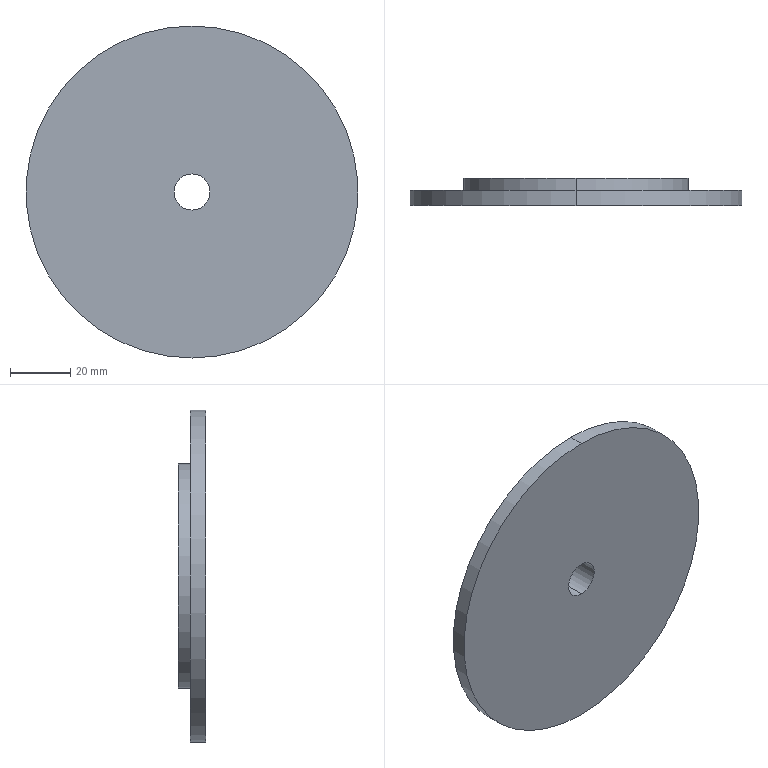Part | NX | features BREP 1 | 1 solid | 9 faces | box 110 x 9 x 110 mm | volume 63935 mm3 | cylinder 6 | plane 3 | commonest cylinder face diameters 12 x2 74.5 x2 110 x2
STEP:
#1=CARTESIAN_POINT('',(0.,6.5,37.25));
#2=VERTEX_POINT('',#1);
#3=CARTESIAN_POINT('',(0.,6.5,-37.25));
#4=VERTEX_POINT('',#3);
#5=CARTESIAN_POINT('',(0.,6.5,0.));
#6=DIRECTION('',(0.,1.,0.));
#7=DIRECTION('',(0.,0.,1.));
#8=AXIS2_PLACEMENT_3D('',#5,#6,#7);
#9=CIRCLE('',#8,37.25);
#10=EDGE_CURVE('',#2,#4,#9,.T.);
#11=ORIENTED_EDGE('',*,*,#10,.F.);
#12=CARTESIAN_POINT('',(0.,2.5,37.25));
#13=VERTEX_POINT('',#12);
#14=CARTESIAN_POINT('',(0.,6.5,37.25));
#15=DIRECTION('',(0.,-1.,0.));
#16=VECTOR('',#15,1000.);
#17=LINE('',#14,#16);
#18=EDGE_CURVE('',#13,#2,#17,.F.);
#19=ORIENTED_EDGE('',*,*,#18,.F.);
#20=CARTESIAN_POINT('',(0.,2.5,-37.25));
#21=VERTEX_POINT('',#20);
#22=CARTESIAN_POINT('',(0.,2.5,0.));
#23=DIRECTION('',(0.,1.,0.));
#24=DIRECTION('',(0.,0.,1.));
#25=AXIS2_PLACEMENT_3D('',#22,#23,#24);
#26=CIRCLE('',#25,37.25);
#27=EDGE_CURVE('',#13,#21,#26,.T.);
#28=ORIENTED_EDGE('',*,*,#27,.T.);
#29=CARTESIAN_POINT('',(0.,6.5,-37.25));
#30=DIRECTION('',(0.,-1.,0.));
#31=VECTOR('',#30,1000.);
#32=LINE('',#29,#31);
#33=EDGE_CURVE('',#21,#4,#32,.F.);
#34=ORIENTED_EDGE('',*,*,#33,.T.);
#35=EDGE_LOOP('',(#11,#19,#28,#34));
#36=FACE_BOUND('',#35,.T.);
#37=CARTESIAN_POINT('',(0.,6.5,0.));
#38=DIRECTION('',(0.,-1.,0.));
#39=DIRECTION('',(0.,0.,1.));
#40=AXIS2_PLACEMENT_3D('',#37,#38,#39);
#41=CYLINDRICAL_SURFACE('',#40,37.25);
#42=ADVANCED_FACE('',(#36),#41,.T.);
#43=CARTESIAN_POINT('',(0.,6.5,-6.));
#44=VERTEX_POINT('',#43);
#45=CARTESIAN_POINT('',(0.,6.5,6.));
#46=VERTEX_POINT('',#45);
#47=CARTESIAN_POINT('',(0.,6.5,0.));
#48=DIRECTION('',(0.,1.,0.));
#49=DIRECTION('',(0.,0.,1.));
#50=AXIS2_PLACEMENT_3D('',#47,#48,#49);
#51=CIRCLE('',#50,6.);
#52=EDGE_CURVE('',#44,#46,#51,.T.);
#53=ORIENTED_EDGE('',*,*,#52,.T.);
#54=CARTESIAN_POINT('',(0.,-2.5,6.));
#55=VERTEX_POINT('',#54);
#56=CARTESIAN_POINT('',(0.,2.5,6.));
#57=DIRECTION('',(0.,-1.,0.));
#58=VECTOR('',#57,1000.);
#59=LINE('',#56,#58);
#60=EDGE_CURVE('',#55,#46,#59,.F.);
#61=ORIENTED_EDGE('',*,*,#60,.F.);
#62=CARTESIAN_POINT('',(0.,-2.5,-6.));
#63=VERTEX_POINT('',#62);
#64=CARTESIAN_POINT('',(0.,-2.5,0.));
#65=DIRECTION('',(0.,1.,0.));
#66=DIRECTION('',(0.,0.,1.));
#67=AXIS2_PLACEMENT_3D('',#64,#65,#66);
#68=CIRCLE('',#67,6.);
#69=EDGE_CURVE('',#63,#55,#68,.T.);
#70=ORIENTED_EDGE('',*,*,#69,.F.);
#71=CARTESIAN_POINT('',(0.,2.5,-6.));
#72=DIRECTION('',(0.,-1.,0.));
#73=VECTOR('',#72,1000.);
#74=LINE('',#71,#73);
#75=EDGE_CURVE('',#63,#44,#74,.F.);
#76=ORIENTED_EDGE('',*,*,#75,.T.);
#77=EDGE_LOOP('',(#53,#61,#70,#76));
#78=FACE_BOUND('',#77,.T.);
#79=CARTESIAN_POINT('',(0.,2.5,0.));
#80=DIRECTION('',(0.,-1.,0.));
#81=DIRECTION('',(0.,0.,1.));
#82=AXIS2_PLACEMENT_3D('',#79,#80,#81);
#83=CYLINDRICAL_SURFACE('',#82,6.);
#84=ADVANCED_FACE('',(#78),#83,.F.);
#85=CARTESIAN_POINT('',(0.,2.5,55.));
#86=VERTEX_POINT('',#85);
#87=CARTESIAN_POINT('',(0.,2.5,-55.));
#88=VERTEX_POINT('',#87);
#89=CARTESIAN_POINT('',(0.,2.5,0.));
#90=DIRECTION('',(0.,1.,0.));
#91=DIRECTION('',(0.,0.,1.));
#92=AXIS2_PLACEMENT_3D('',#89,#90,#91);
#93=CIRCLE('',#92,55.);
#94=EDGE_CURVE('',#86,#88,#93,.T.);
#95=ORIENTED_EDGE('',*,*,#94,.F.);
#96=CARTESIAN_POINT('',(0.,-2.5,55.));
#97=VERTEX_POINT('',#96);
#98=CARTESIAN_POINT('',(0.,2.5,55.));
#99=DIRECTION('',(0.,-1.,0.));
#100=VECTOR('',#99,1000.);
#101=LINE('',#98,#100);
#102=EDGE_CURVE('',#97,#86,#101,.F.);
#103=ORIENTED_EDGE('',*,*,#102,.F.);
#104=CARTESIAN_POINT('',(0.,-2.5,-55.));
#105=VERTEX_POINT('',#104);
#106=CARTESIAN_POINT('',(0.,-2.5,0.));
#107=DIRECTION('',(0.,1.,0.));
#108=DIRECTION('',(0.,0.,1.));
#109=AXIS2_PLACEMENT_3D('',#106,#107,#108);
#110=CIRCLE('',#109,55.);
#111=EDGE_CURVE('',#97,#105,#110,.T.);
#112=ORIENTED_EDGE('',*,*,#111,.T.);
#113=CARTESIAN_POINT('',(0.,2.5,-55.));
#114=DIRECTION('',(0.,-1.,0.));
#115=VECTOR('',#114,1000.);
#116=LINE('',#113,#115);
#117=EDGE_CURVE('',#105,#88,#116,.F.);
#118=ORIENTED_EDGE('',*,*,#117,.T.);
#119=EDGE_LOOP('',(#95,#103,#112,#118));
#120=FACE_BOUND('',#119,.T.);
#121=CARTESIAN_POINT('',(0.,2.5,0.));
#122=DIRECTION('',(0.,-1.,0.));
#123=DIRECTION('',(0.,0.,1.));
#124=AXIS2_PLACEMENT_3D('',#121,#122,#123);
#125=CYLINDRICAL_SURFACE('',#124,55.);
#126=ADVANCED_FACE('',(#120),#125,.T.);
#127=CARTESIAN_POINT('',(0.,2.5,0.));
#128=DIRECTION('',(0.,1.,0.));
#129=DIRECTION('',(0.,0.,1.));
#130=AXIS2_PLACEMENT_3D('',#127,#128,#129);
#131=CIRCLE('',#130,55.);
#132=EDGE_CURVE('',#88,#86,#131,.T.);
#133=ORIENTED_EDGE('',*,*,#132,.T.);
#134=ORIENTED_EDGE('',*,*,#94,.T.);
#135=EDGE_LOOP('',(#133,#134));
#136=FACE_BOUND('',#135,.T.);
#137=CARTESIAN_POINT('',(0.,2.5,0.));
#138=DIRECTION('',(0.,1.,0.));
#139=DIRECTION('',(0.,0.,1.));
#140=AXIS2_PLACEMENT_3D('',#137,#138,#139);
#141=CIRCLE('',#140,37.25);
#142=EDGE_CURVE('',#21,#13,#141,.T.);
#143=ORIENTED_EDGE('',*,*,#142,.F.);
#144=ORIENTED_EDGE('',*,*,#27,.F.);
#145=EDGE_LOOP('',(#143,#144));
#146=FACE_BOUND('',#145,.T.);
#147=CARTESIAN_POINT('',(0.,2.5,0.));
#148=DIRECTION('',(0.,1.,0.));
#149=DIRECTION('',(0.,0.,-1.));
#150=AXIS2_PLACEMENT_3D('',#147,#148,#149);
#151=PLANE('',#150);
#152=ADVANCED_FACE('',(#136,#146),#151,.T.);
#153=CARTESIAN_POINT('',(0.,-2.5,0.));
#154=DIRECTION('',(0.,1.,0.));
#155=DIRECTION('',(0.,0.,1.));
#156=AXIS2_PLACEMENT_3D('',#153,#154,#155);
#157=CIRCLE('',#156,55.);
#158=EDGE_CURVE('',#105,#97,#157,.T.);
#159=ORIENTED_EDGE('',*,*,#158,.F.);
#160=ORIENTED_EDGE('',*,*,#111,.F.);
#161=EDGE_LOOP('',(#159,#160));
#162=FACE_BOUND('',#161,.T.);
#163=ORIENTED_EDGE('',*,*,#69,.T.);
#164=CARTESIAN_POINT('',(0.,-2.5,0.));
#165=DIRECTION('',(0.,1.,0.));
#166=DIRECTION('',(0.,0.,1.));
#167=AXIS2_PLACEMENT_3D('',#164,#165,#166);
#168=CIRCLE('',#167,6.);
#169=EDGE_CURVE('',#55,#63,#168,.T.);
#170=ORIENTED_EDGE('',*,*,#169,.T.);
#171=EDGE_LOOP('',(#163,#170));
#172=FACE_BOUND('',#171,.T.);
#173=CARTESIAN_POINT('',(0.,-2.5,0.));
#174=DIRECTION('',(0.,1.,0.));
#175=DIRECTION('',(0.,0.,-1.));
#176=AXIS2_PLACEMENT_3D('',#173,#174,#175);
#177=PLANE('',#176);
#178=ADVANCED_FACE('',(#162,#172),#177,.F.);
#179=ORIENTED_EDGE('',*,*,#102,.T.);
#180=ORIENTED_EDGE('',*,*,#132,.F.);
#181=ORIENTED_EDGE('',*,*,#117,.F.);
#182=ORIENTED_EDGE('',*,*,#158,.T.);
#183=EDGE_LOOP('',(#179,#180,#181,#182));
#184=FACE_BOUND('',#183,.T.);
#185=CARTESIAN_POINT('',(0.,2.5,0.));
#186=DIRECTION('',(0.,-1.,0.));
#187=DIRECTION('',(0.,0.,1.));
#188=AXIS2_PLACEMENT_3D('',#185,#186,#187);
#189=CYLINDRICAL_SURFACE('',#188,55.);
#190=ADVANCED_FACE('',(#184),#189,.T.);
#191=ORIENTED_EDGE('',*,*,#60,.T.);
#192=CARTESIAN_POINT('',(0.,6.5,0.));
#193=DIRECTION('',(0.,1.,0.));
#194=DIRECTION('',(0.,0.,1.));
#195=AXIS2_PLACEMENT_3D('',#192,#193,#194);
#196=CIRCLE('',#195,6.);
#197=EDGE_CURVE('',#46,#44,#196,.T.);
#198=ORIENTED_EDGE('',*,*,#197,.T.);
#199=ORIENTED_EDGE('',*,*,#75,.F.);
#200=ORIENTED_EDGE('',*,*,#169,.F.);
#201=EDGE_LOOP('',(#191,#198,#199,#200));
#202=FACE_BOUND('',#201,.T.);
#203=CARTESIAN_POINT('',(0.,2.5,0.));
#204=DIRECTION('',(0.,-1.,0.));
#205=DIRECTION('',(0.,0.,1.));
#206=AXIS2_PLACEMENT_3D('',#203,#204,#205);
#207=CYLINDRICAL_SURFACE('',#206,6.);
#208=ADVANCED_FACE('',(#202),#207,.F.);
#209=CARTESIAN_POINT('',(0.,6.5,0.));
#210=DIRECTION('',(0.,1.,0.));
#211=DIRECTION('',(0.,0.,1.));
#212=AXIS2_PLACEMENT_3D('',#209,#210,#211);
#213=CIRCLE('',#212,37.25);
#214=EDGE_CURVE('',#4,#2,#213,.T.);
#215=ORIENTED_EDGE('',*,*,#214,.T.);
#216=ORIENTED_EDGE('',*,*,#10,.T.);
#217=EDGE_LOOP('',(#215,#216));
#218=FACE_BOUND('',#217,.T.);
#219=ORIENTED_EDGE('',*,*,#52,.F.);
#220=ORIENTED_EDGE('',*,*,#197,.F.);
#221=EDGE_LOOP('',(#219,#220));
#222=FACE_BOUND('',#221,.T.);
#223=CARTESIAN_POINT('',(0.,6.5,0.));
#224=DIRECTION('',(0.,1.,0.));
#225=DIRECTION('',(0.,0.,-1.));
#226=AXIS2_PLACEMENT_3D('',#223,#224,#225);
#227=PLANE('',#226);
#228=ADVANCED_FACE('',(#218,#222),#227,.T.);
#229=ORIENTED_EDGE('',*,*,#18,.T.);
#230=ORIENTED_EDGE('',*,*,#214,.F.);
#231=ORIENTED_EDGE('',*,*,#33,.F.);
#232=ORIENTED_EDGE('',*,*,#142,.T.);
#233=EDGE_LOOP('',(#229,#230,#231,#232));
#234=FACE_BOUND('',#233,.T.);
#235=CARTESIAN_POINT('',(0.,6.5,0.));
#236=DIRECTION('',(0.,-1.,0.));
#237=DIRECTION('',(0.,0.,1.));
#238=AXIS2_PLACEMENT_3D('',#235,#236,#237);
#239=CYLINDRICAL_SURFACE('',#238,37.25);
#240=ADVANCED_FACE('',(#234),#239,.T.);
#241=CLOSED_SHELL('',(#42,#84,#126,#152,#178,#190,#208,#228,#240));
#242=MANIFOLD_SOLID_BREP('',#241);
#243=(LENGTH_UNIT()NAMED_UNIT(*)SI_UNIT(.MILLI.,.METRE.));
#244=UNCERTAINTY_MEASURE_WITH_UNIT(LENGTH_MEASURE(0.00001),#243,'','');
#245=(NAMED_UNIT(*)PLANE_ANGLE_UNIT()SI_UNIT($,.RADIAN.));
#246=(NAMED_UNIT(*)SI_UNIT($,.STERADIAN.)SOLID_ANGLE_UNIT());
#247=(GEOMETRIC_REPRESENTATION_CONTEXT(3)GLOBAL_UNCERTAINTY_ASSIGNED_CONTEXT((#244))GLOBAL_UNIT_ASSIGNED_CONTEXT((#243,#245,#246))REPRESENTATION_CONTEXT('',''));
#248=ADVANCED_BREP_SHAPE_REPRESENTATION('',(#242),#247);